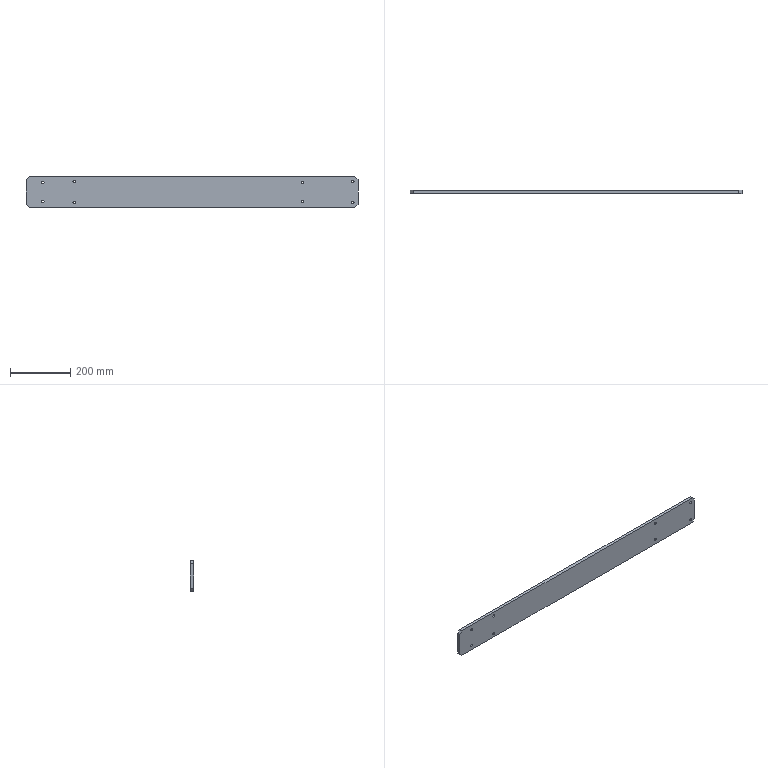Part | NX | features BREP 1 | 1 solid | 26 faces | box 1100 x 10 x 100 mm | volume 1093186 mm3 | cylinder 16 | plane 10 | commonest cylinder face diameters 8.5 x8 9 x8
STEP:
#1=CARTESIAN_POINT('',(366.,10.,27.25));
#2=VERTEX_POINT('',#1);
#3=CARTESIAN_POINT('',(366.,10.,35.75));
#4=VERTEX_POINT('',#3);
#5=CARTESIAN_POINT('',(366.,10.,31.5));
#6=DIRECTION('',(0.,1.,0.));
#7=DIRECTION('',(0.,0.,1.));
#8=AXIS2_PLACEMENT_3D('',#5,#6,#7);
#9=CIRCLE('',#8,4.25);
#10=EDGE_CURVE('',#2,#4,#9,.T.);
#11=ORIENTED_EDGE('',*,*,#10,.T.);
#12=CARTESIAN_POINT('',(366.,0.,35.75));
#13=VERTEX_POINT('',#12);
#14=CARTESIAN_POINT('',(366.,0.,35.75));
#15=DIRECTION('',(0.,-1.,0.));
#16=VECTOR('',#15,1000.);
#17=LINE('',#14,#16);
#18=EDGE_CURVE('',#4,#13,#17,.T.);
#19=ORIENTED_EDGE('',*,*,#18,.T.);
#20=CARTESIAN_POINT('',(366.,0.,27.25));
#21=VERTEX_POINT('',#20);
#22=CARTESIAN_POINT('',(366.,0.,31.5));
#23=DIRECTION('',(0.,-1.,0.));
#24=DIRECTION('',(0.,0.,-1.));
#25=AXIS2_PLACEMENT_3D('',#22,#23,#24);
#26=CIRCLE('',#25,4.25);
#27=EDGE_CURVE('',#13,#21,#26,.T.);
#28=ORIENTED_EDGE('',*,*,#27,.T.);
#29=CARTESIAN_POINT('',(366.,0.,27.25));
#30=DIRECTION('',(0.,-1.,0.));
#31=VECTOR('',#30,1000.);
#32=LINE('',#29,#31);
#33=EDGE_CURVE('',#2,#21,#32,.T.);
#34=ORIENTED_EDGE('',*,*,#33,.F.);
#35=EDGE_LOOP('',(#11,#19,#28,#34));
#36=FACE_BOUND('',#35,.T.);
#37=CARTESIAN_POINT('',(366.,0.,31.5));
#38=DIRECTION('',(0.,-1.,0.));
#39=DIRECTION('',(0.,0.,-1.));
#40=AXIS2_PLACEMENT_3D('',#37,#38,#39);
#41=CYLINDRICAL_SURFACE('',#40,4.25);
#42=ADVANCED_FACE('',(#36),#41,.F.);
#43=CARTESIAN_POINT('',(366.,10.,-35.75));
#44=VERTEX_POINT('',#43);
#45=CARTESIAN_POINT('',(366.,10.,-27.25));
#46=VERTEX_POINT('',#45);
#47=CARTESIAN_POINT('',(366.,10.,-31.5));
#48=DIRECTION('',(0.,1.,0.));
#49=DIRECTION('',(0.,0.,1.));
#50=AXIS2_PLACEMENT_3D('',#47,#48,#49);
#51=CIRCLE('',#50,4.25);
#52=EDGE_CURVE('',#44,#46,#51,.T.);
#53=ORIENTED_EDGE('',*,*,#52,.T.);
#54=CARTESIAN_POINT('',(366.,0.,-27.25));
#55=VERTEX_POINT('',#54);
#56=CARTESIAN_POINT('',(366.,0.,-27.25));
#57=DIRECTION('',(0.,-1.,0.));
#58=VECTOR('',#57,1000.);
#59=LINE('',#56,#58);
#60=EDGE_CURVE('',#46,#55,#59,.T.);
#61=ORIENTED_EDGE('',*,*,#60,.T.);
#62=CARTESIAN_POINT('',(366.,0.,-35.75));
#63=VERTEX_POINT('',#62);
#64=CARTESIAN_POINT('',(366.,0.,-31.5));
#65=DIRECTION('',(0.,-1.,0.));
#66=DIRECTION('',(0.,0.,-1.));
#67=AXIS2_PLACEMENT_3D('',#64,#65,#66);
#68=CIRCLE('',#67,4.25);
#69=EDGE_CURVE('',#55,#63,#68,.T.);
#70=ORIENTED_EDGE('',*,*,#69,.T.);
#71=CARTESIAN_POINT('',(366.,0.,-35.75));
#72=DIRECTION('',(0.,-1.,0.));
#73=VECTOR('',#72,1000.);
#74=LINE('',#71,#73);
#75=EDGE_CURVE('',#44,#63,#74,.T.);
#76=ORIENTED_EDGE('',*,*,#75,.F.);
#77=EDGE_LOOP('',(#53,#61,#70,#76));
#78=FACE_BOUND('',#77,.T.);
#79=CARTESIAN_POINT('',(366.,0.,-31.5));
#80=DIRECTION('',(0.,-1.,0.));
#81=DIRECTION('',(0.,0.,-1.));
#82=AXIS2_PLACEMENT_3D('',#79,#80,#81);
#83=CYLINDRICAL_SURFACE('',#82,4.25);
#84=ADVANCED_FACE('',(#78),#83,.F.);
#85=CARTESIAN_POINT('',(-494.,10.,27.25));
#86=VERTEX_POINT('',#85);
#87=CARTESIAN_POINT('',(-494.,10.,35.75));
#88=VERTEX_POINT('',#87);
#89=CARTESIAN_POINT('',(-494.,10.,31.5));
#90=DIRECTION('',(0.,1.,0.));
#91=DIRECTION('',(0.,0.,1.));
#92=AXIS2_PLACEMENT_3D('',#89,#90,#91);
#93=CIRCLE('',#92,4.25);
#94=EDGE_CURVE('',#86,#88,#93,.T.);
#95=ORIENTED_EDGE('',*,*,#94,.T.);
#96=CARTESIAN_POINT('',(-494.,0.,35.75));
#97=VERTEX_POINT('',#96);
#98=CARTESIAN_POINT('',(-494.,0.,35.75));
#99=DIRECTION('',(0.,-1.,0.));
#100=VECTOR('',#99,1000.);
#101=LINE('',#98,#100);
#102=EDGE_CURVE('',#88,#97,#101,.T.);
#103=ORIENTED_EDGE('',*,*,#102,.T.);
#104=CARTESIAN_POINT('',(-494.,0.,27.25));
#105=VERTEX_POINT('',#104);
#106=CARTESIAN_POINT('',(-494.,0.,31.5));
#107=DIRECTION('',(0.,-1.,0.));
#108=DIRECTION('',(0.,0.,-1.));
#109=AXIS2_PLACEMENT_3D('',#106,#107,#108);
#110=CIRCLE('',#109,4.25);
#111=EDGE_CURVE('',#97,#105,#110,.T.);
#112=ORIENTED_EDGE('',*,*,#111,.T.);
#113=CARTESIAN_POINT('',(-494.,0.,27.25));
#114=DIRECTION('',(0.,-1.,0.));
#115=VECTOR('',#114,1000.);
#116=LINE('',#113,#115);
#117=EDGE_CURVE('',#86,#105,#116,.T.);
#118=ORIENTED_EDGE('',*,*,#117,.F.);
#119=EDGE_LOOP('',(#95,#103,#112,#118));
#120=FACE_BOUND('',#119,.T.);
#121=CARTESIAN_POINT('',(-494.,0.,31.5));
#122=DIRECTION('',(0.,-1.,0.));
#123=DIRECTION('',(0.,0.,-1.));
#124=AXIS2_PLACEMENT_3D('',#121,#122,#123);
#125=CYLINDRICAL_SURFACE('',#124,4.25);
#126=ADVANCED_FACE('',(#120),#125,.F.);
#127=CARTESIAN_POINT('',(-494.,10.,-35.75));
#128=VERTEX_POINT('',#127);
#129=CARTESIAN_POINT('',(-494.,10.,-27.25));
#130=VERTEX_POINT('',#129);
#131=CARTESIAN_POINT('',(-494.,10.,-31.5));
#132=DIRECTION('',(0.,1.,0.));
#133=DIRECTION('',(0.,0.,1.));
#134=AXIS2_PLACEMENT_3D('',#131,#132,#133);
#135=CIRCLE('',#134,4.25);
#136=EDGE_CURVE('',#128,#130,#135,.T.);
#137=ORIENTED_EDGE('',*,*,#136,.T.);
#138=CARTESIAN_POINT('',(-494.,0.,-27.25));
#139=VERTEX_POINT('',#138);
#140=CARTESIAN_POINT('',(-494.,0.,-27.25));
#141=DIRECTION('',(0.,-1.,0.));
#142=VECTOR('',#141,1000.);
#143=LINE('',#140,#142);
#144=EDGE_CURVE('',#130,#139,#143,.T.);
#145=ORIENTED_EDGE('',*,*,#144,.T.);
#146=CARTESIAN_POINT('',(-494.,0.,-35.75));
#147=VERTEX_POINT('',#146);
#148=CARTESIAN_POINT('',(-494.,0.,-31.5));
#149=DIRECTION('',(0.,-1.,0.));
#150=DIRECTION('',(0.,0.,-1.));
#151=AXIS2_PLACEMENT_3D('',#148,#149,#150);
#152=CIRCLE('',#151,4.25);
#153=EDGE_CURVE('',#139,#147,#152,.T.);
#154=ORIENTED_EDGE('',*,*,#153,.T.);
#155=CARTESIAN_POINT('',(-494.,0.,-35.75));
#156=DIRECTION('',(0.,-1.,0.));
#157=VECTOR('',#156,1000.);
#158=LINE('',#155,#157);
#159=EDGE_CURVE('',#128,#147,#158,.T.);
#160=ORIENTED_EDGE('',*,*,#159,.F.);
#161=EDGE_LOOP('',(#137,#145,#154,#160));
#162=FACE_BOUND('',#161,.T.);
#163=CARTESIAN_POINT('',(-494.,0.,-31.5));
#164=DIRECTION('',(0.,-1.,0.));
#165=DIRECTION('',(0.,0.,-1.));
#166=AXIS2_PLACEMENT_3D('',#163,#164,#165);
#167=CYLINDRICAL_SURFACE('',#166,4.25);
#168=ADVANCED_FACE('',(#162),#167,.F.);
#169=CARTESIAN_POINT('',(-390.,0.,-39.5));
#170=VERTEX_POINT('',#169);
#171=CARTESIAN_POINT('',(-390.,0.,-30.5));
#172=VERTEX_POINT('',#171);
#173=CARTESIAN_POINT('',(-390.,0.,-35.));
#174=DIRECTION('',(0.,1.,0.));
#175=DIRECTION('',(0.,0.,1.));
#176=AXIS2_PLACEMENT_3D('',#173,#174,#175);
#177=CIRCLE('',#176,4.5);
#178=EDGE_CURVE('',#170,#172,#177,.T.);
#179=ORIENTED_EDGE('',*,*,#178,.F.);
#180=CARTESIAN_POINT('',(-390.,10.,-39.5));
#181=VERTEX_POINT('',#180);
#182=CARTESIAN_POINT('',(-390.,10.,-39.5));
#183=DIRECTION('',(0.,1.,0.));
#184=VECTOR('',#183,1000.);
#185=LINE('',#182,#184);
#186=EDGE_CURVE('',#181,#170,#185,.F.);
#187=ORIENTED_EDGE('',*,*,#186,.F.);
#188=CARTESIAN_POINT('',(-390.,10.,-30.5));
#189=VERTEX_POINT('',#188);
#190=CARTESIAN_POINT('',(-390.,10.,-35.));
#191=DIRECTION('',(0.,1.,0.));
#192=DIRECTION('',(0.,0.,1.));
#193=AXIS2_PLACEMENT_3D('',#190,#191,#192);
#194=CIRCLE('',#193,4.5);
#195=EDGE_CURVE('',#181,#189,#194,.T.);
#196=ORIENTED_EDGE('',*,*,#195,.T.);
#197=CARTESIAN_POINT('',(-390.,10.,-30.5));
#198=DIRECTION('',(0.,1.,0.));
#199=VECTOR('',#198,1000.);
#200=LINE('',#197,#199);
#201=EDGE_CURVE('',#189,#172,#200,.F.);
#202=ORIENTED_EDGE('',*,*,#201,.T.);
#203=EDGE_LOOP('',(#179,#187,#196,#202));
#204=FACE_BOUND('',#203,.T.);
#205=CARTESIAN_POINT('',(-390.,10.,-35.));
#206=DIRECTION('',(0.,1.,0.));
#207=DIRECTION('',(0.,0.,1.));
#208=AXIS2_PLACEMENT_3D('',#205,#206,#207);
#209=CYLINDRICAL_SURFACE('',#208,4.5);
#210=ADVANCED_FACE('',(#204),#209,.F.);
#211=CARTESIAN_POINT('',(-390.,0.,30.5));
#212=VERTEX_POINT('',#211);
#213=CARTESIAN_POINT('',(-390.,0.,39.5));
#214=VERTEX_POINT('',#213);
#215=CARTESIAN_POINT('',(-390.,0.,35.));
#216=DIRECTION('',(0.,1.,0.));
#217=DIRECTION('',(0.,0.,1.));
#218=AXIS2_PLACEMENT_3D('',#215,#216,#217);
#219=CIRCLE('',#218,4.5);
#220=EDGE_CURVE('',#212,#214,#219,.T.);
#221=ORIENTED_EDGE('',*,*,#220,.F.);
#222=CARTESIAN_POINT('',(-390.,10.,30.5));
#223=VERTEX_POINT('',#222);
#224=CARTESIAN_POINT('',(-390.,10.,30.5));
#225=DIRECTION('',(0.,1.,0.));
#226=VECTOR('',#225,1000.);
#227=LINE('',#224,#226);
#228=EDGE_CURVE('',#223,#212,#227,.F.);
#229=ORIENTED_EDGE('',*,*,#228,.F.);
#230=CARTESIAN_POINT('',(-390.,10.,39.5));
#231=VERTEX_POINT('',#230);
#232=CARTESIAN_POINT('',(-390.,10.,35.));
#233=DIRECTION('',(0.,1.,0.));
#234=DIRECTION('',(0.,0.,1.));
#235=AXIS2_PLACEMENT_3D('',#232,#233,#234);
#236=CIRCLE('',#235,4.5);
#237=EDGE_CURVE('',#223,#231,#236,.T.);
#238=ORIENTED_EDGE('',*,*,#237,.T.);
#239=CARTESIAN_POINT('',(-390.,10.,39.5));
#240=DIRECTION('',(0.,1.,0.));
#241=VECTOR('',#240,1000.);
#242=LINE('',#239,#241);
#243=EDGE_CURVE('',#231,#214,#242,.F.);
#244=ORIENTED_EDGE('',*,*,#243,.T.);
#245=EDGE_LOOP('',(#221,#229,#238,#244));
#246=FACE_BOUND('',#245,.T.);
#247=CARTESIAN_POINT('',(-390.,10.,35.));
#248=DIRECTION('',(0.,1.,0.));
#249=DIRECTION('',(0.,0.,1.));
#250=AXIS2_PLACEMENT_3D('',#247,#248,#249);
#251=CYLINDRICAL_SURFACE('',#250,4.5);
#252=ADVANCED_FACE('',(#246),#251,.F.);
#253=CARTESIAN_POINT('',(532.5,0.,-39.5));
#254=VERTEX_POINT('',#253);
#255=CARTESIAN_POINT('',(532.5,0.,-30.5));
#256=VERTEX_POINT('',#255);
#257=CARTESIAN_POINT('',(532.5,0.,-35.));
#258=DIRECTION('',(0.,1.,0.));
#259=DIRECTION('',(0.,0.,1.));
#260=AXIS2_PLACEMENT_3D('',#257,#258,#259);
#261=CIRCLE('',#260,4.5);
#262=EDGE_CURVE('',#254,#256,#261,.T.);
#263=ORIENTED_EDGE('',*,*,#262,.F.);
#264=CARTESIAN_POINT('',(532.5,10.,-39.5));
#265=VERTEX_POINT('',#264);
#266=CARTESIAN_POINT('',(532.5,10.,-39.5));
#267=DIRECTION('',(0.,1.,0.));
#268=VECTOR('',#267,1000.);
#269=LINE('',#266,#268);
#270=EDGE_CURVE('',#265,#254,#269,.F.);
#271=ORIENTED_EDGE('',*,*,#270,.F.);
#272=CARTESIAN_POINT('',(532.5,10.,-30.5));
#273=VERTEX_POINT('',#272);
#274=CARTESIAN_POINT('',(532.5,10.,-35.));
#275=DIRECTION('',(0.,1.,0.));
#276=DIRECTION('',(0.,0.,1.));
#277=AXIS2_PLACEMENT_3D('',#274,#275,#276);
#278=CIRCLE('',#277,4.5);
#279=EDGE_CURVE('',#265,#273,#278,.T.);
#280=ORIENTED_EDGE('',*,*,#279,.T.);
#281=CARTESIAN_POINT('',(532.5,10.,-30.5));
#282=DIRECTION('',(0.,1.,0.));
#283=VECTOR('',#282,1000.);
#284=LINE('',#281,#283);
#285=EDGE_CURVE('',#273,#256,#284,.F.);
#286=ORIENTED_EDGE('',*,*,#285,.T.);
#287=EDGE_LOOP('',(#263,#271,#280,#286));
#288=FACE_BOUND('',#287,.T.);
#289=CARTESIAN_POINT('',(532.5,10.,-35.));
#290=DIRECTION('',(0.,1.,0.));
#291=DIRECTION('',(0.,0.,1.));
#292=AXIS2_PLACEMENT_3D('',#289,#290,#291);
#293=CYLINDRICAL_SURFACE('',#292,4.5);
#294=ADVANCED_FACE('',(#288),#293,.F.);
#295=CARTESIAN_POINT('',(532.5,0.,30.5));
#296=VERTEX_POINT('',#295);
#297=CARTESIAN_POINT('',(532.5,0.,39.5));
#298=VERTEX_POINT('',#297);
#299=CARTESIAN_POINT('',(532.5,0.,35.));
#300=DIRECTION('',(0.,1.,0.));
#301=DIRECTION('',(0.,0.,1.));
#302=AXIS2_PLACEMENT_3D('',#299,#300,#301);
#303=CIRCLE('',#302,4.5);
#304=EDGE_CURVE('',#296,#298,#303,.T.);
#305=ORIENTED_EDGE('',*,*,#304,.F.);
#306=CARTESIAN_POINT('',(532.5,10.,30.5));
#307=VERTEX_POINT('',#306);
#308=CARTESIAN_POINT('',(532.5,10.,30.5));
#309=DIRECTION('',(0.,1.,0.));
#310=VECTOR('',#309,1000.);
#311=LINE('',#308,#310);
#312=EDGE_CURVE('',#307,#296,#311,.F.);
#313=ORIENTED_EDGE('',*,*,#312,.F.);
#314=CARTESIAN_POINT('',(532.5,10.,39.5));
#315=VERTEX_POINT('',#314);
#316=CARTESIAN_POINT('',(532.5,10.,35.));
#317=DIRECTION('',(0.,1.,0.));
#318=DIRECTION('',(0.,0.,1.));
#319=AXIS2_PLACEMENT_3D('',#316,#317,#318);
#320=CIRCLE('',#319,4.5);
#321=EDGE_CURVE('',#307,#315,#320,.T.);
#322=ORIENTED_EDGE('',*,*,#321,.T.);
#323=CARTESIAN_POINT('',(532.5,10.,39.5));
#324=DIRECTION('',(0.,1.,0.));
#325=VECTOR('',#324,1000.);
#326=LINE('',#323,#325);
#327=EDGE_CURVE('',#315,#298,#326,.F.);
#328=ORIENTED_EDGE('',*,*,#327,.T.);
#329=EDGE_LOOP('',(#305,#313,#322,#328));
#330=FACE_BOUND('',#329,.T.);
#331=CARTESIAN_POINT('',(532.5,10.,35.));
#332=DIRECTION('',(0.,1.,0.));
#333=DIRECTION('',(0.,0.,1.));
#334=AXIS2_PLACEMENT_3D('',#331,#332,#333);
#335=CYLINDRICAL_SURFACE('',#334,4.5);
#336=ADVANCED_FACE('',(#330),#335,.F.);
#337=CARTESIAN_POINT('',(550.,10.,40.));
#338=VERTEX_POINT('',#337);
#339=CARTESIAN_POINT('',(550.,10.,-40.));
#340=VERTEX_POINT('',#339);
#341=CARTESIAN_POINT('',(550.,10.,-50.));
#342=DIRECTION('',(0.,0.,-1.));
#343=VECTOR('',#342,1000.);
#344=LINE('',#341,#343);
#345=EDGE_CURVE('',#338,#340,#344,.T.);
#346=ORIENTED_EDGE('',*,*,#345,.F.);
#347=CARTESIAN_POINT('',(550.,0.,40.));
#348=VERTEX_POINT('',#347);
#349=CARTESIAN_POINT('',(550.,10.,40.));
#350=DIRECTION('',(0.,-1.,0.));
#351=VECTOR('',#350,1000.);
#352=LINE('',#349,#351);
#353=EDGE_CURVE('',#338,#348,#352,.T.);
#354=ORIENTED_EDGE('',*,*,#353,.T.);
#355=CARTESIAN_POINT('',(550.,0.,-40.));
#356=VERTEX_POINT('',#355);
#357=CARTESIAN_POINT('',(550.,0.,-50.));
#358=DIRECTION('',(0.,0.,-1.));
#359=VECTOR('',#358,1000.);
#360=LINE('',#357,#359);
#361=EDGE_CURVE('',#348,#356,#360,.T.);
#362=ORIENTED_EDGE('',*,*,#361,.T.);
#363=CARTESIAN_POINT('',(550.,10.,-40.));
#364=DIRECTION('',(0.,1.,0.));
#365=VECTOR('',#364,1000.);
#366=LINE('',#363,#365);
#367=EDGE_CURVE('',#356,#340,#366,.T.);
#368=ORIENTED_EDGE('',*,*,#367,.T.);
#369=EDGE_LOOP('',(#346,#354,#362,#368));
#370=FACE_BOUND('',#369,.T.);
#371=CARTESIAN_POINT('',(550.,10.,-50.));
#372=DIRECTION('',(-1.,0.,0.));
#373=DIRECTION('',(0.,0.,1.));
#374=AXIS2_PLACEMENT_3D('',#371,#372,#373);
#375=PLANE('',#374);
#376=ADVANCED_FACE('',(#370),#375,.F.);
#377=CARTESIAN_POINT('',(540.,10.,-50.));
#378=VERTEX_POINT('',#377);
#379=CARTESIAN_POINT('',(-540.,10.,-50.));
#380=VERTEX_POINT('',#379);
#381=CARTESIAN_POINT('',(-550.,10.,-50.));
#382=DIRECTION('',(-1.,0.,0.));
#383=VECTOR('',#382,1000.);
#384=LINE('',#381,#383);
#385=EDGE_CURVE('',#378,#380,#384,.T.);
#386=ORIENTED_EDGE('',*,*,#385,.F.);
#387=CARTESIAN_POINT('',(540.,0.,-50.));
#388=VERTEX_POINT('',#387);
#389=CARTESIAN_POINT('',(540.,10.,-50.));
#390=DIRECTION('',(0.,-1.,0.));
#391=VECTOR('',#390,1000.);
#392=LINE('',#389,#391);
#393=EDGE_CURVE('',#378,#388,#392,.T.);
#394=ORIENTED_EDGE('',*,*,#393,.T.);
#395=CARTESIAN_POINT('',(-540.,0.,-50.));
#396=VERTEX_POINT('',#395);
#397=CARTESIAN_POINT('',(-550.,0.,-50.));
#398=DIRECTION('',(-1.,0.,0.));
#399=VECTOR('',#398,1000.);
#400=LINE('',#397,#399);
#401=EDGE_CURVE('',#388,#396,#400,.T.);
#402=ORIENTED_EDGE('',*,*,#401,.T.);
#403=CARTESIAN_POINT('',(-540.,10.,-50.));
#404=DIRECTION('',(0.,1.,0.));
#405=VECTOR('',#404,1000.);
#406=LINE('',#403,#405);
#407=EDGE_CURVE('',#396,#380,#406,.T.);
#408=ORIENTED_EDGE('',*,*,#407,.T.);
#409=EDGE_LOOP('',(#386,#394,#402,#408));
#410=FACE_BOUND('',#409,.T.);
#411=CARTESIAN_POINT('',(-550.,10.,-50.));
#412=DIRECTION('',(0.,0.,1.));
#413=DIRECTION('',(1.,0.,0.));
#414=AXIS2_PLACEMENT_3D('',#411,#412,#413);
#415=PLANE('',#414);
#416=ADVANCED_FACE('',(#410),#415,.F.);
#417=CARTESIAN_POINT('',(-550.,0.,-40.));
#418=VERTEX_POINT('',#417);
#419=CARTESIAN_POINT('',(-550.,0.,40.));
#420=VERTEX_POINT('',#419);
#421=CARTESIAN_POINT('',(-550.,0.,-50.));
#422=DIRECTION('',(0.,0.,1.));
#423=VECTOR('',#422,1000.);
#424=LINE('',#421,#423);
#425=EDGE_CURVE('',#418,#420,#424,.T.);
#426=ORIENTED_EDGE('',*,*,#425,.T.);
#427=CARTESIAN_POINT('',(-550.,10.,40.));
#428=VERTEX_POINT('',#427);
#429=CARTESIAN_POINT('',(-550.,10.,40.));
#430=DIRECTION('',(0.,1.,0.));
#431=VECTOR('',#430,1000.);
#432=LINE('',#429,#431);
#433=EDGE_CURVE('',#420,#428,#432,.T.);
#434=ORIENTED_EDGE('',*,*,#433,.T.);
#435=CARTESIAN_POINT('',(-550.,10.,-40.));
#436=VERTEX_POINT('',#435);
#437=CARTESIAN_POINT('',(-550.,10.,-50.));
#438=DIRECTION('',(0.,0.,1.));
#439=VECTOR('',#438,1000.);
#440=LINE('',#437,#439);
#441=EDGE_CURVE('',#436,#428,#440,.T.);
#442=ORIENTED_EDGE('',*,*,#441,.F.);
#443=CARTESIAN_POINT('',(-550.,10.,-40.));
#444=DIRECTION('',(0.,-1.,0.));
#445=VECTOR('',#444,1000.);
#446=LINE('',#443,#445);
#447=EDGE_CURVE('',#436,#418,#446,.T.);
#448=ORIENTED_EDGE('',*,*,#447,.T.);
#449=EDGE_LOOP('',(#426,#434,#442,#448));
#450=FACE_BOUND('',#449,.T.);
#451=CARTESIAN_POINT('',(-550.,10.,-50.));
#452=DIRECTION('',(1.,0.,0.));
#453=DIRECTION('',(0.,1.,0.));
#454=AXIS2_PLACEMENT_3D('',#451,#452,#453);
#455=PLANE('',#454);
#456=ADVANCED_FACE('',(#450),#455,.F.);
#457=CARTESIAN_POINT('',(-540.,0.,50.));
#458=VERTEX_POINT('',#457);
#459=CARTESIAN_POINT('',(540.,0.,50.));
#460=VERTEX_POINT('',#459);
#461=CARTESIAN_POINT('',(-550.,0.,50.));
#462=DIRECTION('',(1.,0.,0.));
#463=VECTOR('',#462,1000.);
#464=LINE('',#461,#463);
#465=EDGE_CURVE('',#458,#460,#464,.T.);
#466=ORIENTED_EDGE('',*,*,#465,.T.);
#467=CARTESIAN_POINT('',(540.,10.,50.));
#468=VERTEX_POINT('',#467);
#469=CARTESIAN_POINT('',(540.,10.,50.));
#470=DIRECTION('',(0.,1.,0.));
#471=VECTOR('',#470,1000.);
#472=LINE('',#469,#471);
#473=EDGE_CURVE('',#460,#468,#472,.T.);
#474=ORIENTED_EDGE('',*,*,#473,.T.);
#475=CARTESIAN_POINT('',(-540.,10.,50.));
#476=VERTEX_POINT('',#475);
#477=CARTESIAN_POINT('',(-550.,10.,50.));
#478=DIRECTION('',(1.,0.,0.));
#479=VECTOR('',#478,1000.);
#480=LINE('',#477,#479);
#481=EDGE_CURVE('',#476,#468,#480,.T.);
#482=ORIENTED_EDGE('',*,*,#481,.F.);
#483=CARTESIAN_POINT('',(-540.,10.,50.));
#484=DIRECTION('',(0.,-1.,0.));
#485=VECTOR('',#484,1000.);
#486=LINE('',#483,#485);
#487=EDGE_CURVE('',#476,#458,#486,.T.);
#488=ORIENTED_EDGE('',*,*,#487,.T.);
#489=EDGE_LOOP('',(#466,#474,#482,#488));
#490=FACE_BOUND('',#489,.T.);
#491=CARTESIAN_POINT('',(-550.,10.,50.));
#492=DIRECTION('',(0.,0.,-1.));
#493=DIRECTION('',(0.,-1.,0.));
#494=AXIS2_PLACEMENT_3D('',#491,#492,#493);
#495=PLANE('',#494);
#496=ADVANCED_FACE('',(#490),#495,.F.);
#497=ORIENTED_EDGE('',*,*,#481,.T.);
#498=CARTESIAN_POINT('',(295.,10.,295.));
#499=DIRECTION('',(0.7071,0.,-0.7071));
#500=VECTOR('',#499,1000.);
#501=LINE('',#498,#500);
#502=EDGE_CURVE('',#468,#338,#501,.T.);
#503=ORIENTED_EDGE('',*,*,#502,.T.);
#504=ORIENTED_EDGE('',*,*,#345,.T.);
#505=CARTESIAN_POINT('',(295.,10.,-295.));
#506=DIRECTION('',(-0.7071,0.,-0.7071));
#507=VECTOR('',#506,1000.);
#508=LINE('',#505,#507);
#509=EDGE_CURVE('',#340,#378,#508,.T.);
#510=ORIENTED_EDGE('',*,*,#509,.T.);
#511=ORIENTED_EDGE('',*,*,#385,.T.);
#512=CARTESIAN_POINT('',(-295.,10.,-295.));
#513=DIRECTION('',(-0.7071,0.,0.7071));
#514=VECTOR('',#513,1000.);
#515=LINE('',#512,#514);
#516=EDGE_CURVE('',#380,#436,#515,.T.);
#517=ORIENTED_EDGE('',*,*,#516,.T.);
#518=ORIENTED_EDGE('',*,*,#441,.T.);
#519=CARTESIAN_POINT('',(-295.,10.,295.));
#520=DIRECTION('',(0.7071,0.,0.7071));
#521=VECTOR('',#520,1000.);
#522=LINE('',#519,#521);
#523=EDGE_CURVE('',#428,#476,#522,.T.);
#524=ORIENTED_EDGE('',*,*,#523,.T.);
#525=EDGE_LOOP('',(#497,#503,#504,#510,#511,#517,#518,#524));
#526=FACE_BOUND('',#525,.T.);
#527=ORIENTED_EDGE('',*,*,#10,.F.);
#528=CARTESIAN_POINT('',(366.,10.,31.5));
#529=DIRECTION('',(0.,1.,0.));
#530=DIRECTION('',(0.,0.,1.));
#531=AXIS2_PLACEMENT_3D('',#528,#529,#530);
#532=CIRCLE('',#531,4.25);
#533=EDGE_CURVE('',#4,#2,#532,.T.);
#534=ORIENTED_EDGE('',*,*,#533,.F.);
#535=EDGE_LOOP('',(#527,#534));
#536=FACE_BOUND('',#535,.T.);
#537=ORIENTED_EDGE('',*,*,#52,.F.);
#538=CARTESIAN_POINT('',(366.,10.,-31.5));
#539=DIRECTION('',(0.,1.,0.));
#540=DIRECTION('',(0.,0.,1.));
#541=AXIS2_PLACEMENT_3D('',#538,#539,#540);
#542=CIRCLE('',#541,4.25);
#543=EDGE_CURVE('',#46,#44,#542,.T.);
#544=ORIENTED_EDGE('',*,*,#543,.F.);
#545=EDGE_LOOP('',(#537,#544));
#546=FACE_BOUND('',#545,.T.);
#547=ORIENTED_EDGE('',*,*,#94,.F.);
#548=CARTESIAN_POINT('',(-494.,10.,31.5));
#549=DIRECTION('',(0.,1.,0.));
#550=DIRECTION('',(0.,0.,1.));
#551=AXIS2_PLACEMENT_3D('',#548,#549,#550);
#552=CIRCLE('',#551,4.25);
#553=EDGE_CURVE('',#88,#86,#552,.T.);
#554=ORIENTED_EDGE('',*,*,#553,.F.);
#555=EDGE_LOOP('',(#547,#554));
#556=FACE_BOUND('',#555,.T.);
#557=ORIENTED_EDGE('',*,*,#136,.F.);
#558=CARTESIAN_POINT('',(-494.,10.,-31.5));
#559=DIRECTION('',(0.,1.,0.));
#560=DIRECTION('',(0.,0.,1.));
#561=AXIS2_PLACEMENT_3D('',#558,#559,#560);
#562=CIRCLE('',#561,4.25);
#563=EDGE_CURVE('',#130,#128,#562,.T.);
#564=ORIENTED_EDGE('',*,*,#563,.F.);
#565=EDGE_LOOP('',(#557,#564));
#566=FACE_BOUND('',#565,.T.);
#567=CARTESIAN_POINT('',(-390.,10.,-35.));
#568=DIRECTION('',(0.,1.,0.));
#569=DIRECTION('',(0.,0.,1.));
#570=AXIS2_PLACEMENT_3D('',#567,#568,#569);
#571=CIRCLE('',#570,4.5);
#572=EDGE_CURVE('',#189,#181,#571,.T.);
#573=ORIENTED_EDGE('',*,*,#572,.F.);
#574=ORIENTED_EDGE('',*,*,#195,.F.);
#575=EDGE_LOOP('',(#573,#574));
#576=FACE_BOUND('',#575,.T.);
#577=CARTESIAN_POINT('',(-390.,10.,35.));
#578=DIRECTION('',(0.,1.,0.));
#579=DIRECTION('',(0.,0.,1.));
#580=AXIS2_PLACEMENT_3D('',#577,#578,#579);
#581=CIRCLE('',#580,4.5);
#582=EDGE_CURVE('',#231,#223,#581,.T.);
#583=ORIENTED_EDGE('',*,*,#582,.F.);
#584=ORIENTED_EDGE('',*,*,#237,.F.);
#585=EDGE_LOOP('',(#583,#584));
#586=FACE_BOUND('',#585,.T.);
#587=CARTESIAN_POINT('',(532.5,10.,-35.));
#588=DIRECTION('',(0.,1.,0.));
#589=DIRECTION('',(0.,0.,1.));
#590=AXIS2_PLACEMENT_3D('',#587,#588,#589);
#591=CIRCLE('',#590,4.5);
#592=EDGE_CURVE('',#273,#265,#591,.T.);
#593=ORIENTED_EDGE('',*,*,#592,.F.);
#594=ORIENTED_EDGE('',*,*,#279,.F.);
#595=EDGE_LOOP('',(#593,#594));
#596=FACE_BOUND('',#595,.T.);
#597=CARTESIAN_POINT('',(532.5,10.,35.));
#598=DIRECTION('',(0.,1.,0.));
#599=DIRECTION('',(0.,0.,1.));
#600=AXIS2_PLACEMENT_3D('',#597,#598,#599);
#601=CIRCLE('',#600,4.5);
#602=EDGE_CURVE('',#315,#307,#601,.T.);
#603=ORIENTED_EDGE('',*,*,#602,.F.);
#604=ORIENTED_EDGE('',*,*,#321,.F.);
#605=EDGE_LOOP('',(#603,#604));
#606=FACE_BOUND('',#605,.T.);
#607=CARTESIAN_POINT('',(0.,10.,0.));
#608=DIRECTION('',(0.,1.,0.));
#609=DIRECTION('',(1.,0.,0.));
#610=AXIS2_PLACEMENT_3D('',#607,#608,#609);
#611=PLANE('',#610);
#612=ADVANCED_FACE('',(#526,#536,#546,#556,#566,#576,#586,#596,#606),#611,.T.);
#613=ORIENTED_EDGE('',*,*,#361,.F.);
#614=CARTESIAN_POINT('',(550.,0.,40.));
#615=DIRECTION('',(-0.7071,0.,0.7071));
#616=VECTOR('',#615,1000.);
#617=LINE('',#614,#616);
#618=EDGE_CURVE('',#348,#460,#617,.T.);
#619=ORIENTED_EDGE('',*,*,#618,.T.);
#620=ORIENTED_EDGE('',*,*,#465,.F.);
#621=CARTESIAN_POINT('',(-540.,0.,50.));
#622=DIRECTION('',(-0.7071,0.,-0.7071));
#623=VECTOR('',#622,1000.);
#624=LINE('',#621,#623);
#625=EDGE_CURVE('',#458,#420,#624,.T.);
#626=ORIENTED_EDGE('',*,*,#625,.T.);
#627=ORIENTED_EDGE('',*,*,#425,.F.);
#628=CARTESIAN_POINT('',(-550.,0.,-40.));
#629=DIRECTION('',(0.7071,0.,-0.7071));
#630=VECTOR('',#629,1000.);
#631=LINE('',#628,#630);
#632=EDGE_CURVE('',#418,#396,#631,.T.);
#633=ORIENTED_EDGE('',*,*,#632,.T.);
#634=ORIENTED_EDGE('',*,*,#401,.F.);
#635=CARTESIAN_POINT('',(540.,0.,-50.));
#636=DIRECTION('',(0.7071,0.,0.7071));
#637=VECTOR('',#636,1000.);
#638=LINE('',#635,#637);
#639=EDGE_CURVE('',#388,#356,#638,.T.);
#640=ORIENTED_EDGE('',*,*,#639,.T.);
#641=EDGE_LOOP('',(#613,#619,#620,#626,#627,#633,#634,#640));
#642=FACE_BOUND('',#641,.T.);
#643=CARTESIAN_POINT('',(366.,0.,31.5));
#644=DIRECTION('',(0.,-1.,0.));
#645=DIRECTION('',(0.,0.,-1.));
#646=AXIS2_PLACEMENT_3D('',#643,#644,#645);
#647=CIRCLE('',#646,4.25);
#648=EDGE_CURVE('',#21,#13,#647,.T.);
#649=ORIENTED_EDGE('',*,*,#648,.F.);
#650=ORIENTED_EDGE('',*,*,#27,.F.);
#651=EDGE_LOOP('',(#649,#650));
#652=FACE_BOUND('',#651,.T.);
#653=CARTESIAN_POINT('',(366.,0.,-31.5));
#654=DIRECTION('',(0.,-1.,0.));
#655=DIRECTION('',(0.,0.,-1.));
#656=AXIS2_PLACEMENT_3D('',#653,#654,#655);
#657=CIRCLE('',#656,4.25);
#658=EDGE_CURVE('',#63,#55,#657,.T.);
#659=ORIENTED_EDGE('',*,*,#658,.F.);
#660=ORIENTED_EDGE('',*,*,#69,.F.);
#661=EDGE_LOOP('',(#659,#660));
#662=FACE_BOUND('',#661,.T.);
#663=CARTESIAN_POINT('',(-494.,0.,31.5));
#664=DIRECTION('',(0.,-1.,0.));
#665=DIRECTION('',(0.,0.,-1.));
#666=AXIS2_PLACEMENT_3D('',#663,#664,#665);
#667=CIRCLE('',#666,4.25);
#668=EDGE_CURVE('',#105,#97,#667,.T.);
#669=ORIENTED_EDGE('',*,*,#668,.F.);
#670=ORIENTED_EDGE('',*,*,#111,.F.);
#671=EDGE_LOOP('',(#669,#670));
#672=FACE_BOUND('',#671,.T.);
#673=CARTESIAN_POINT('',(-494.,0.,-31.5));
#674=DIRECTION('',(0.,-1.,0.));
#675=DIRECTION('',(0.,0.,-1.));
#676=AXIS2_PLACEMENT_3D('',#673,#674,#675);
#677=CIRCLE('',#676,4.25);
#678=EDGE_CURVE('',#147,#139,#677,.T.);
#679=ORIENTED_EDGE('',*,*,#678,.F.);
#680=ORIENTED_EDGE('',*,*,#153,.F.);
#681=EDGE_LOOP('',(#679,#680));
#682=FACE_BOUND('',#681,.T.);
#683=CARTESIAN_POINT('',(-390.,0.,-35.));
#684=DIRECTION('',(0.,1.,0.));
#685=DIRECTION('',(0.,0.,1.));
#686=AXIS2_PLACEMENT_3D('',#683,#684,#685);
#687=CIRCLE('',#686,4.5);
#688=EDGE_CURVE('',#172,#170,#687,.T.);
#689=ORIENTED_EDGE('',*,*,#688,.T.);
#690=ORIENTED_EDGE('',*,*,#178,.T.);
#691=EDGE_LOOP('',(#689,#690));
#692=FACE_BOUND('',#691,.T.);
#693=CARTESIAN_POINT('',(-390.,0.,35.));
#694=DIRECTION('',(0.,1.,0.));
#695=DIRECTION('',(0.,0.,1.));
#696=AXIS2_PLACEMENT_3D('',#693,#694,#695);
#697=CIRCLE('',#696,4.5);
#698=EDGE_CURVE('',#214,#212,#697,.T.);
#699=ORIENTED_EDGE('',*,*,#698,.T.);
#700=ORIENTED_EDGE('',*,*,#220,.T.);
#701=EDGE_LOOP('',(#699,#700));
#702=FACE_BOUND('',#701,.T.);
#703=CARTESIAN_POINT('',(532.5,0.,-35.));
#704=DIRECTION('',(0.,1.,0.));
#705=DIRECTION('',(0.,0.,1.));
#706=AXIS2_PLACEMENT_3D('',#703,#704,#705);
#707=CIRCLE('',#706,4.5);
#708=EDGE_CURVE('',#256,#254,#707,.T.);
#709=ORIENTED_EDGE('',*,*,#708,.T.);
#710=ORIENTED_EDGE('',*,*,#262,.T.);
#711=EDGE_LOOP('',(#709,#710));
#712=FACE_BOUND('',#711,.T.);
#713=CARTESIAN_POINT('',(532.5,0.,35.));
#714=DIRECTION('',(0.,1.,0.));
#715=DIRECTION('',(0.,0.,1.));
#716=AXIS2_PLACEMENT_3D('',#713,#714,#715);
#717=CIRCLE('',#716,4.5);
#718=EDGE_CURVE('',#298,#296,#717,.T.);
#719=ORIENTED_EDGE('',*,*,#718,.T.);
#720=ORIENTED_EDGE('',*,*,#304,.T.);
#721=EDGE_LOOP('',(#719,#720));
#722=FACE_BOUND('',#721,.T.);
#723=CARTESIAN_POINT('',(0.,0.,0.));
#724=DIRECTION('',(0.,1.,0.));
#725=DIRECTION('',(1.,0.,0.));
#726=AXIS2_PLACEMENT_3D('',#723,#724,#725);
#727=PLANE('',#726);
#728=ADVANCED_FACE('',(#642,#652,#662,#672,#682,#692,#702,#712,#722),#727,.F.);
#729=ORIENTED_EDGE('',*,*,#312,.T.);
#730=ORIENTED_EDGE('',*,*,#718,.F.);
#731=ORIENTED_EDGE('',*,*,#327,.F.);
#732=ORIENTED_EDGE('',*,*,#602,.T.);
#733=EDGE_LOOP('',(#729,#730,#731,#732));
#734=FACE_BOUND('',#733,.T.);
#735=CARTESIAN_POINT('',(532.5,10.,35.));
#736=DIRECTION('',(0.,1.,0.));
#737=DIRECTION('',(0.,0.,1.));
#738=AXIS2_PLACEMENT_3D('',#735,#736,#737);
#739=CYLINDRICAL_SURFACE('',#738,4.5);
#740=ADVANCED_FACE('',(#734),#739,.F.);
#741=ORIENTED_EDGE('',*,*,#270,.T.);
#742=ORIENTED_EDGE('',*,*,#708,.F.);
#743=ORIENTED_EDGE('',*,*,#285,.F.);
#744=ORIENTED_EDGE('',*,*,#592,.T.);
#745=EDGE_LOOP('',(#741,#742,#743,#744));
#746=FACE_BOUND('',#745,.T.);
#747=CARTESIAN_POINT('',(532.5,10.,-35.));
#748=DIRECTION('',(0.,1.,0.));
#749=DIRECTION('',(0.,0.,1.));
#750=AXIS2_PLACEMENT_3D('',#747,#748,#749);
#751=CYLINDRICAL_SURFACE('',#750,4.5);
#752=ADVANCED_FACE('',(#746),#751,.F.);
#753=ORIENTED_EDGE('',*,*,#228,.T.);
#754=ORIENTED_EDGE('',*,*,#698,.F.);
#755=ORIENTED_EDGE('',*,*,#243,.F.);
#756=ORIENTED_EDGE('',*,*,#582,.T.);
#757=EDGE_LOOP('',(#753,#754,#755,#756));
#758=FACE_BOUND('',#757,.T.);
#759=CARTESIAN_POINT('',(-390.,10.,35.));
#760=DIRECTION('',(0.,1.,0.));
#761=DIRECTION('',(0.,0.,1.));
#762=AXIS2_PLACEMENT_3D('',#759,#760,#761);
#763=CYLINDRICAL_SURFACE('',#762,4.5);
#764=ADVANCED_FACE('',(#758),#763,.F.);
#765=ORIENTED_EDGE('',*,*,#186,.T.);
#766=ORIENTED_EDGE('',*,*,#688,.F.);
#767=ORIENTED_EDGE('',*,*,#201,.F.);
#768=ORIENTED_EDGE('',*,*,#572,.T.);
#769=EDGE_LOOP('',(#765,#766,#767,#768));
#770=FACE_BOUND('',#769,.T.);
#771=CARTESIAN_POINT('',(-390.,10.,-35.));
#772=DIRECTION('',(0.,1.,0.));
#773=DIRECTION('',(0.,0.,1.));
#774=AXIS2_PLACEMENT_3D('',#771,#772,#773);
#775=CYLINDRICAL_SURFACE('',#774,4.5);
#776=ADVANCED_FACE('',(#770),#775,.F.);
#777=ORIENTED_EDGE('',*,*,#502,.F.);
#778=ORIENTED_EDGE('',*,*,#473,.F.);
#779=ORIENTED_EDGE('',*,*,#618,.F.);
#780=ORIENTED_EDGE('',*,*,#353,.F.);
#781=EDGE_LOOP('',(#777,#778,#779,#780));
#782=FACE_BOUND('',#781,.T.);
#783=CARTESIAN_POINT('',(550.,10.,40.));
#784=DIRECTION('',(-0.7071,0.,-0.7071));
#785=DIRECTION('',(-0.7071,0.,0.7071));
#786=AXIS2_PLACEMENT_3D('',#783,#784,#785);
#787=PLANE('',#786);
#788=ADVANCED_FACE('',(#782),#787,.F.);
#789=ORIENTED_EDGE('',*,*,#509,.F.);
#790=ORIENTED_EDGE('',*,*,#367,.F.);
#791=ORIENTED_EDGE('',*,*,#639,.F.);
#792=ORIENTED_EDGE('',*,*,#393,.F.);
#793=EDGE_LOOP('',(#789,#790,#791,#792));
#794=FACE_BOUND('',#793,.T.);
#795=CARTESIAN_POINT('',(540.,10.,-50.));
#796=DIRECTION('',(-0.7071,0.,0.7071));
#797=DIRECTION('',(0.,1.,0.));
#798=AXIS2_PLACEMENT_3D('',#795,#796,#797);
#799=PLANE('',#798);
#800=ADVANCED_FACE('',(#794),#799,.F.);
#801=ORIENTED_EDGE('',*,*,#523,.F.);
#802=ORIENTED_EDGE('',*,*,#433,.F.);
#803=ORIENTED_EDGE('',*,*,#625,.F.);
#804=ORIENTED_EDGE('',*,*,#487,.F.);
#805=EDGE_LOOP('',(#801,#802,#803,#804));
#806=FACE_BOUND('',#805,.T.);
#807=CARTESIAN_POINT('',(-540.,10.,50.));
#808=DIRECTION('',(0.7071,0.,-0.7071));
#809=DIRECTION('',(0.,-1.,0.));
#810=AXIS2_PLACEMENT_3D('',#807,#808,#809);
#811=PLANE('',#810);
#812=ADVANCED_FACE('',(#806),#811,.F.);
#813=ORIENTED_EDGE('',*,*,#516,.F.);
#814=ORIENTED_EDGE('',*,*,#407,.F.);
#815=ORIENTED_EDGE('',*,*,#632,.F.);
#816=ORIENTED_EDGE('',*,*,#447,.F.);
#817=EDGE_LOOP('',(#813,#814,#815,#816));
#818=FACE_BOUND('',#817,.T.);
#819=CARTESIAN_POINT('',(-550.,10.,-40.));
#820=DIRECTION('',(0.7071,0.,0.7071));
#821=DIRECTION('',(0.,-1.,0.));
#822=AXIS2_PLACEMENT_3D('',#819,#820,#821);
#823=PLANE('',#822);
#824=ADVANCED_FACE('',(#818),#823,.F.);
#825=ORIENTED_EDGE('',*,*,#144,.F.);
#826=ORIENTED_EDGE('',*,*,#563,.T.);
#827=ORIENTED_EDGE('',*,*,#159,.T.);
#828=ORIENTED_EDGE('',*,*,#678,.T.);
#829=EDGE_LOOP('',(#825,#826,#827,#828));
#830=FACE_BOUND('',#829,.T.);
#831=CARTESIAN_POINT('',(-494.,0.,-31.5));
#832=DIRECTION('',(0.,-1.,0.));
#833=DIRECTION('',(0.,0.,-1.));
#834=AXIS2_PLACEMENT_3D('',#831,#832,#833);
#835=CYLINDRICAL_SURFACE('',#834,4.25);
#836=ADVANCED_FACE('',(#830),#835,.F.);
#837=ORIENTED_EDGE('',*,*,#102,.F.);
#838=ORIENTED_EDGE('',*,*,#553,.T.);
#839=ORIENTED_EDGE('',*,*,#117,.T.);
#840=ORIENTED_EDGE('',*,*,#668,.T.);
#841=EDGE_LOOP('',(#837,#838,#839,#840));
#842=FACE_BOUND('',#841,.T.);
#843=CARTESIAN_POINT('',(-494.,0.,31.5));
#844=DIRECTION('',(0.,-1.,0.));
#845=DIRECTION('',(0.,0.,-1.));
#846=AXIS2_PLACEMENT_3D('',#843,#844,#845);
#847=CYLINDRICAL_SURFACE('',#846,4.25);
#848=ADVANCED_FACE('',(#842),#847,.F.);
#849=ORIENTED_EDGE('',*,*,#60,.F.);
#850=ORIENTED_EDGE('',*,*,#543,.T.);
#851=ORIENTED_EDGE('',*,*,#75,.T.);
#852=ORIENTED_EDGE('',*,*,#658,.T.);
#853=EDGE_LOOP('',(#849,#850,#851,#852));
#854=FACE_BOUND('',#853,.T.);
#855=CARTESIAN_POINT('',(366.,0.,-31.5));
#856=DIRECTION('',(0.,-1.,0.));
#857=DIRECTION('',(0.,0.,-1.));
#858=AXIS2_PLACEMENT_3D('',#855,#856,#857);
#859=CYLINDRICAL_SURFACE('',#858,4.25);
#860=ADVANCED_FACE('',(#854),#859,.F.);
#861=ORIENTED_EDGE('',*,*,#18,.F.);
#862=ORIENTED_EDGE('',*,*,#533,.T.);
#863=ORIENTED_EDGE('',*,*,#33,.T.);
#864=ORIENTED_EDGE('',*,*,#648,.T.);
#865=EDGE_LOOP('',(#861,#862,#863,#864));
#866=FACE_BOUND('',#865,.T.);
#867=CARTESIAN_POINT('',(366.,0.,31.5));
#868=DIRECTION('',(0.,-1.,0.));
#869=DIRECTION('',(0.,0.,-1.));
#870=AXIS2_PLACEMENT_3D('',#867,#868,#869);
#871=CYLINDRICAL_SURFACE('',#870,4.25);
#872=ADVANCED_FACE('',(#866),#871,.F.);
#873=CLOSED_SHELL('',(#42,#84,#126,#168,#210,#252,#294,#336,#376,#416,#456,#496,#612,#728,#740,#752,#764,#776,#788,#800,#812,#824,#836,#848,#860,#872));
#874=MANIFOLD_SOLID_BREP('',#873);
#875=(LENGTH_UNIT()NAMED_UNIT(*)SI_UNIT(.MILLI.,.METRE.));
#876=UNCERTAINTY_MEASURE_WITH_UNIT(LENGTH_MEASURE(0.00001),#875,'','');
#877=(NAMED_UNIT(*)PLANE_ANGLE_UNIT()SI_UNIT($,.RADIAN.));
#878=(NAMED_UNIT(*)SI_UNIT($,.STERADIAN.)SOLID_ANGLE_UNIT());
#879=(GEOMETRIC_REPRESENTATION_CONTEXT(3)GLOBAL_UNCERTAINTY_ASSIGNED_CONTEXT((#876))GLOBAL_UNIT_ASSIGNED_CONTEXT((#875,#877,#878))REPRESENTATION_CONTEXT('',''));
#880=ADVANCED_BREP_SHAPE_REPRESENTATION('',(#874),#879);